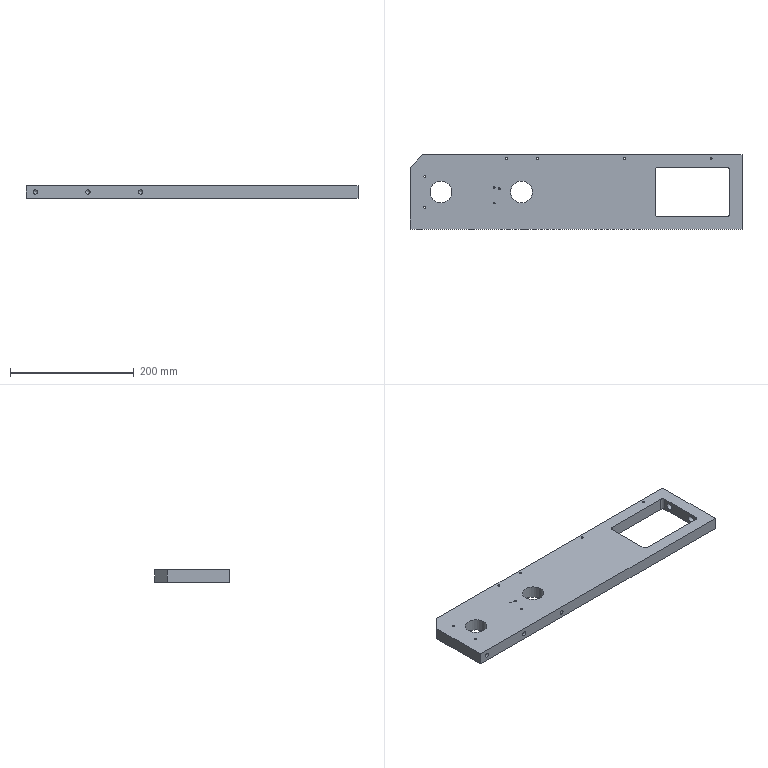CAM job | NX | 3-axis milling, drilling | part box 536 x 120 x 20 mm | stock box 536 x 120 x 20 mm
Tools:
number,name,description,diameter,corner_radius,flute_length,length,flutes
9,D10,平底铣刀-粗,10.0,0.0,35.0,75.0,2
7,D6-J,平底铣刀-精,6.0,0.0,25.0,75.0,2
10,D10-J,平底铣刀-精,10.0,0.0,35.0,75.0,2
2,D6倒角刀,倒角刀,6.0,0.0,3.0,25.0,2
20,M3X0.5,丝锥,2.5,0.0,35.0,50.0,2
21,M4X0.7,丝锥,3.3,0.0,35.0,50.0,2
1,C6定点钻,倒角刀,6.0,0.0,3.0,3.0,2
12,ZT2.6,钻头,2.6,0.0,35.0,50.0,2
13,ZT3.4,钻头,3.4,0.0,35.0,50.0,2
Operations:
program,operation,operation_type,tool,method,geometry_group,spindle_rpm,surface_speed,feed_per_tooth,feed_cut,feed_plunge,cut_length_mm,path_length_mm,cut_time_min,machine_time_min
B,选线往复层切开粗-中_COPY_1,PlanarMilling,D10,分层开粗-切深K-步距G,W-B,3000.0,94.245,0.3333,2000.0,100.0,1712.518,1774.318,0.8563,0.8624
B,钻倒角_3,Operation,D6倒角刀,METHOD,W-B,2000.0,0.0,0.025,100.0,0.0,36.4,685.372,0.364,0.4289
B,C0.3封闭铣廓倒角6X45L_COPY,PlanarMilling,D6倒角刀,爬面_倒角-切深0-步距G,W-B,4000.0,75.398,0.125,1000.0,100.0,1955.162,2836.759,1.955,2.043
B,平面铣精光侧面-中-直线_COPY_1,PlanarMilling,D10-J,侧刃精光-切深K-步距G,W-B,3000.0,94.245,0.1333,800.0,100.0,42.284,102.284,0.0529,0.0589
A,框开粗_1,VolumeBased25DMillingOperation,D10,METHOD,W-A,3000.0,188.0,0.25,2500.0,80.0,53051.926,53649.242,21.221,21.28
A,选线往复层切开粗-中_COPY,PlanarMilling,D10,分层开粗-切深K-步距G,W-A,3000.0,94.245,0.3333,2000.0,100.0,1712.518,1774.318,0.8563,0.8624
A,打点-深0.8,Operation,C6定点钻,NONE,W-A,3000.0,56.0,0.01,60.0,90.0,19.8,722.574,0.33,0.4003
A,盲锥孔-M3螺纹底孔,Operation,ZT2.6,NONE,W-A,2000.0,15.708,0.0125,50.0,90.0,24.0,114.02,0.48,0.489
A,通孔-M4螺纹底孔,Operation,ZT3.4,NONE,W-A,1500.0,15.551,0.02,60.0,90.0,189.0,976.104,3.15,3.229
A,钻倒角_1,Operation,D6倒角刀,METHOD,W-A,4000.0,75.398,0.01,80.0,0.0,9.5,87.179,0.1187,0.1265
A,钻倒角_2,Operation,D6倒角刀,METHOD,W-A,4000.0,75.398,0.01,80.0,0.0,36.4,683.233,0.455,0.5197
A,铣倒角_1,PlanarMilling,D6倒角刀,METHOD,W-A,4000.0,75.398,0.125,1000.0,100.0,225.681,439.82,0.2257,0.2471
A,盲锥孔-攻牙M3,Operation,M3X0.5,METHOD,W-A,600.0,4.712,0.0004,0.5,90.0,15.0,96.02,30.0,30.008
A,通孔-攻牙M4,Operation,M4X0.7,METHOD,W-A,500.0,5.184,0.0007,0.7,90.0,171.5,941.104,245.0,245.077
A,框半精_1,VolumeBased25DMillingOperation,D6-J,METHOD,W-A,3200.0,157.0,0.2,800.0,90.0,1140.532,1739.875,1.428,1.488
A,框精_1,VolumeBased25DMillingOperation,D6-J,METHOD,W-A,3200.0,157.0,0.2,800.0,90.0,570.452,1168.972,0.7141,0.774
A,平面铣精光侧面-中-直线_COPY,PlanarMilling,D10-J,侧刃精光-切深K-步距G,W-A,3000.0,94.245,0.1333,800.0,100.0,42.284,102.284,0.0529,0.0589